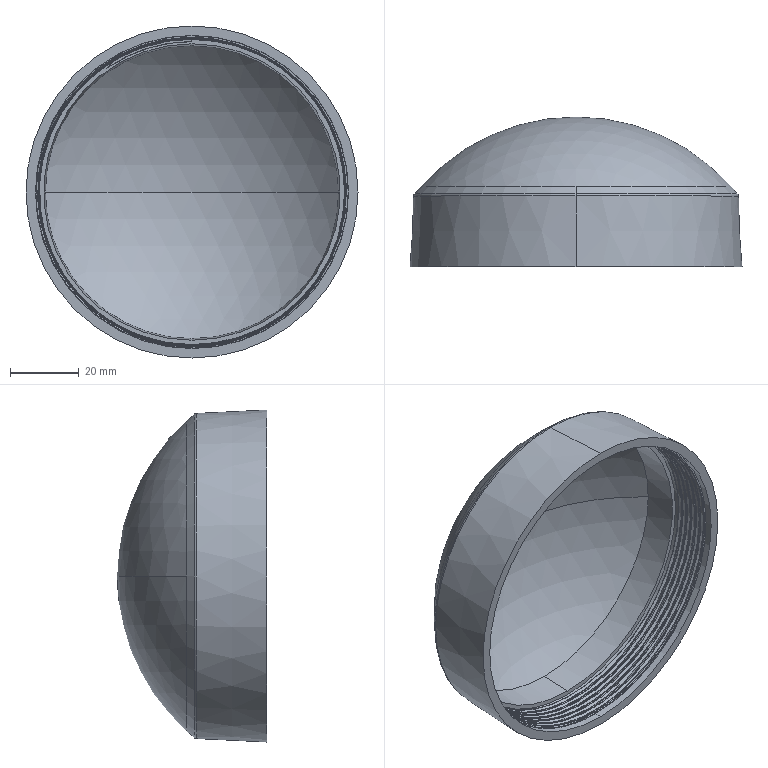Part | SolidWorks | features Helix 1, Revolution 1, SweepCut 1 | 1 solid | 38 faces | box 96.5 x 43.5 x 96.5 mm | volume 37980 mm3 | cone 23 | spline 5 | sphere 4 | plane 4 | torus 2